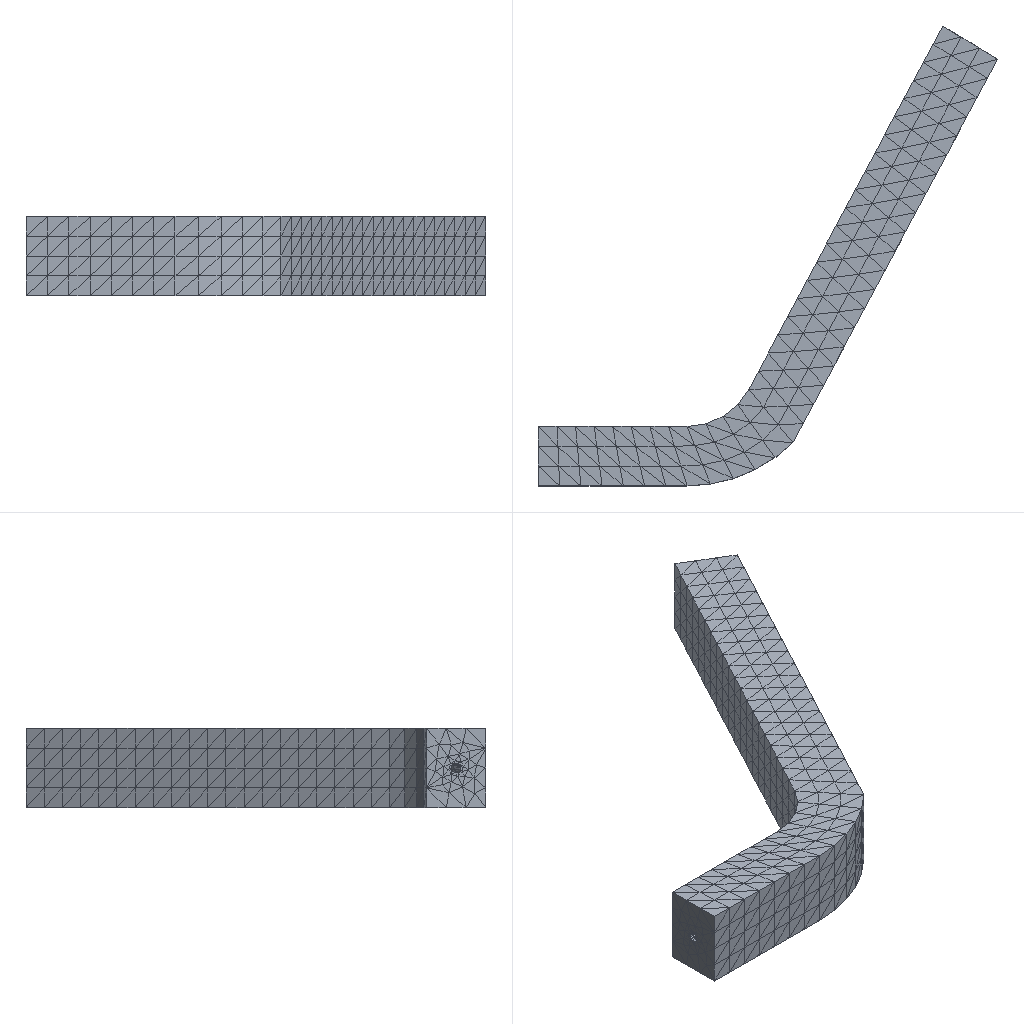Simulation study | abaqus
Set-up summary:
category,name,step,type,value,unit,region
solver,abaqus
solver,version,,,Abaqus/Standard 2020
units,not stated in the deck,,not stated
analysis,deck,,transient,transient
load_step,Step-1,Step-1,transient
load_step,requested,,,1
mesh,nodes,,,8863
mesh,elements,,,21207
element_type,S4R,,shell,2920
element_type,C3D4,,solid,16327
element_type,C3D8,,solid,1960
load,load commands in deck,,count,1
bc,support commands in deck,,count,2
material,CHONG,,in results
material,SOIL,,in results
material,TUBE,,in results
check,setup vs results,,match,"per instance, exact: element labels, types and connectivity; labels of the nodes the elements use; coordinates of those nodes at SINGLE_PRECISION in 2 of 3 instance(s)"
Abaqus input file, long lists of numbers shortened:
*Heading
** Job name: Job-1 Model name: Model-1
** Generated by: Abaqus/CAE 2020
*Preprint, echo=NO, model=NO, history=NO, contact=NO
**
** PARTS
**
*Part, name=chong
*Node
      1,   79.917,   70.314, -0.2075
      2,   79.947,   70.298,  -0.1153
** (2392 more lines like these left out)
*Element, type=C3D8
   1,  121,  214,  215,  138,    7,  100,  101,   24
   2,  122,  123,  146,  213,    8,    9,   32,   99
** (1958 more lines like these left out)
*Nset, nset=Set-1, generate
    1,  2394,     1
*Elset, elset=Set-1, generate
    1,  1960,     1
*Nset, nset=Set-2, generate
    1,  2394,     1
*Elset, elset=Set-2, generate
    1,  1960,     1
** Section: chong
*Solid Section, elset=Set-2, material=chong
,
*End Part
**
*Part, name=soil-delete
*Node
      1,   25.707,  -1.644,           8.
      2,          15.,          -6.,           8.
** (3537 more lines like these left out)
*Element, type=C3D4
    1,  226, 1737, 1738, 1739
    2, 1737, 1740,  438,  436
** (16325 more lines like these left out)
*Nset, nset=Set-1, generate
    1,  3539,     1
*Elset, elset=Set-1, generate
     1,  16327,      1
** Section: soil
*Solid Section, elset=Set-1, material=soil
,
*End Part
**
*Part, name=tube
*Node
      1,   38.406,   12.536, -0.4341
      2,   38.197,   12.672,          0.5
** (2928 more lines like these left out)
*Element, type=S4R
   1,    1,    7,  252,   14
   2,    7,    8,  253,  252
** (2918 more lines like these left out)
*Nset, nset=Set-1, generate
    1,  2930,     1
*Elset, elset=Set-1, generate
    1,  2920,     1
** Section: tube
*Shell Section, elset=Set-1, material=tube
0.01, 5
*End Part
**
**
** ASSEMBLY
**
*Assembly, name=Assembly
**
*Instance, name=soil-delete-1, part=soil-delete
*End Instance
**
*Instance, name=tube-1, part=tube
   -14.447,   -11.422,           4.
*End Instance
**
*Instance, name=chong-1, part=chong
  -36.883,   -33.511,           4.
*End Instance
**
*Node
      1,    43.596,   38.768,           4.
*Nset, nset=Set-1, instance=soil-delete-1
   1,   2,   3,   4,   9,  10,  14,  15,  23,  24,  25,  26,  27,  28,  29,  30
  31,  32,  33,  34,  35,  36,  49,  50,  51,  52,  53,  54,  55,  56,  57,  58
** (9 more lines like these left out)
*Elset, elset=Set-1, instance=soil-delete-1
    81,    98,   396,   701,   845,   892,  1273,  1789,  2345,  2356,  2379,  2423,  2521,  2581,  2591,  2592
  2622,  2642,  2644,  2646,  2669,  2680,  2683,  2695,  2700,  2711,  2712,  2724,  2729,  2745,  2747,  2760
** (14 more lines like these left out)
*Nset, nset=Set-2, instance=soil-delete-1
   1,   2,   3,   4,   5,   6,   7,   8,   9,  10,  11,  12,  13,  14,  15,  16
  23,  24,  25,  26,  30,  31,  32,  33,  37,  38,  39,  43,  44,  45,  49,  50
** (15 more lines like these left out)
*Elset, elset=Set-2, instance=soil-delete-1
    10,   141,   160,   634,   727,  2316,  2329,  2383,  2409,  2425,  2446,  2449,  2469,  2502,  2507,  2510
  2515,  2523,  2531,  2542,  2561,  2572,  2575,  2583,  2593,  2600,  2660,  2685,  2690,  2700,  2704,  2723
** (22 more lines like these left out)
*Nset, nset=Set-4
 1,
*Nset, nset=Set-7
 1,
*Nset, nset=Set-8
 1,
*Nset, nset=Set-9, instance=chong-1, generate
    1,  2394,     1
*Nset, nset=Set-9
 1,
*Elset, elset=Set-9, instance=chong-1, generate
    1,  1960,     1
*Nset, nset=Set-10, instance=chong-1, generate
 2281,  2394,     1
*Elset, elset=Set-10, instance=chong-1, generate
 1863,  1960,     1
*Nset, nset=b_Set-5, instance=chong-1, generate
    1,  2394,     1
*Elset, elset=b_Set-5, instance=chong-1, generate
    1,  1960,     1
*Nset, nset=m_Set-3
 1,
*Nset, nset=_PickedSet26, internal
 1,
*Elset, elset=_Surf-6_S1, internal, instance=chong-1, generate
 1863,  1960,     1
*Surface, type=ELEMENT, name=Surf-6
_Surf-6_S1, S1
*Elset, elset=_Surf-12_S1, internal, instance=chong-1, generate
 1863,  1960,     1
*Surface, type=ELEMENT, name=Surf-12
_Surf-12_S1, S1
*Elset, elset=_m_Surf-3_SPOS, internal, instance=tube-1, generate
    1,  2920,     1
*Surface, type=ELEMENT, name=m_Surf-3
_m_Surf-3_SPOS, SPOS
*Elset, elset=_m_Surf-7_S6, internal, instance=chong-1
    1,   15,   22,   24,   99,  113,  120,  122,  197,  211,  218,  220,  295,  309,  316,  318
  393,  407,  414,  416,  491,  505,  512,  514,  589,  603,  610,  612,  687,  701,  708,  710
** (3 more lines like these left out)
*Elset, elset=_m_Surf-7_S3, internal, instance=chong-1
    2,    3,    4,    9,   12,   21,   26,   27,   31,   33,   39,   40,   44,   88,   90,  100
  101,  102,  107,  110,  119,  124,  125,  129,  131,  137,  138,  142,  186,  188,  198,  199
** (17 more lines like these left out)
*Elset, elset=_m_Surf-7_S4, internal, instance=chong-1
    5,    6,   25,   43,   54,  103,  104,  123,  141,  152,  201,  202,  221,  239,  250,  299
  300,  319,  337,  348,  397,  398,  417,  435,  446,  495,  496,  515,  533,  544,  593,  594
** (5 more lines like these left out)
*Elset, elset=_m_Surf-7_S5, internal, instance=chong-1
   20,   23,   28,   46,   56,   57,  118,  121,  126,  144,  154,  155,  216,  219,  224,  242
  252,  253,  314,  317,  322,  340,  350,  351,  412,  415,  420,  438,  448,  449,  510,  513
** (6 more lines like these left out)
*Surface, type=ELEMENT, name=m_Surf-7
_m_Surf-7_S6, S6
_m_Surf-7_S3, S3
_m_Surf-7_S4, S4
_m_Surf-7_S5, S5
*Elset, elset=_m_Surf-9_S6, internal, instance=chong-1
    1,   15,   22,   24,   99,  113,  120,  122,  197,  211,  218,  220,  295,  309,  316,  318
  393,  407,  414,  416,  491,  505,  512,  514,  589,  603,  610,  612,  687,  701,  708,  710
** (3 more lines like these left out)
*Elset, elset=_m_Surf-9_S3, internal, instance=chong-1
    2,    3,    4,    9,   12,   21,   26,   27,   31,   33,   39,   40,   44,   88,   90,  100
  101,  102,  107,  110,  119,  124,  125,  129,  131,  137,  138,  142,  186,  188,  198,  199
** (17 more lines like these left out)
*Elset, elset=_m_Surf-9_S4, internal, instance=chong-1
    5,    6,   25,   43,   54,  103,  104,  123,  141,  152,  201,  202,  221,  239,  250,  299
  300,  319,  337,  348,  397,  398,  417,  435,  446,  495,  496,  515,  533,  544,  593,  594
** (5 more lines like these left out)
*Elset, elset=_m_Surf-9_S5, internal, instance=chong-1
   20,   23,   28,   46,   56,   57,  118,  121,  126,  144,  154,  155,  216,  219,  224,  242
  252,  253,  314,  317,  322,  340,  350,  351,  412,  415,  420,  438,  448,  449,  510,  513
** (6 more lines like these left out)
*Surface, type=ELEMENT, name=m_Surf-9
_m_Surf-9_S6, S6
_m_Surf-9_S3, S3
_m_Surf-9_S4, S4
_m_Surf-9_S5, S5
*Elset, elset=_s_Surf-1_S4, internal, instance=soil-delete-1
   353,   354,   411,   600,  1045,  1799,  2111,  2165,  2408,  2628,  2755,  3114,  3390,  3399,  3863,  4025
  4148,  4152,  4155,  4516,  4592,  4598,  4867,  4878,  5204,  5264,  5514,  5578,  5588,  5632,  5656,  5686
** (8 more lines like these left out)
*Elset, elset=_s_Surf-1_S3, internal, instance=soil-delete-1
   188,   220,   544,   547,   557,   573,   609,   667,   721,   772,   809,  1021,  1056,  1163,  1184,  1210
  1242,  1291,  1376,  1426,  1904,  1910,  1956,  2163,  2173,  2290,  2360,  2372,  2385,  2397,  2399,  2407
** (131 more lines like these left out)
*Elset, elset=_s_Surf-1_S2, internal, instance=soil-delete-1
   259,   452,   463,  1039,  2512,  2587,  3238,  3459,  4406,  4449,  4641,  5482,  5559,  5655,  5682,  5709
  5844,  5845,  5931,  5998,  6223,  6487,  6607,  6654,  6656,  6877,  6907,  6958,  7062,  7117,  7549,  7899
** (3 more lines like these left out)
*Elset, elset=_s_Surf-1_S1, internal, instance=soil-delete-1
   275,   592,   610,  1227,  1656,  1668,  2450,  2630,  2728,  2895,  3482,  3792,  4225,  4760,  5383,  5666
  5700,  5853,  6283,  6494,  6699,  6726,  6953,  7164,  7395,  7554,  7582,  7583,  7620,  7642,  7643,  7647
** (3 more lines like these left out)
*Surface, type=ELEMENT, name=s_Surf-1
_s_Surf-1_S4, S4
_s_Surf-1_S3, S3
_s_Surf-1_S2, S2
_s_Surf-1_S1, S1
*Elset, elset=_s_Surf-3_S4, internal, instance=soil-delete-1
   353,   354,   411,   600,  1045,  1799,  2111,  2165,  2408,  2628,  2755,  3114,  3390,  3399,  3863,  4025
  4148,  4152,  4155,  4516,  4592,  4598,  4867,  4878,  5204,  5264,  5514,  5578,  5588,  5632,  5656,  5686
** (8 more lines like these left out)
*Elset, elset=_s_Surf-3_S3, internal, instance=soil-delete-1
   188,   220,   544,   547,   557,   573,   609,   667,   721,   772,   809,  1021,  1056,  1163,  1184,  1210
  1242,  1291,  1376,  1426,  1904,  1910,  1956,  2163,  2173,  2290,  2360,  2372,  2385,  2397,  2399,  2407
** (131 more lines like these left out)
*Elset, elset=_s_Surf-3_S2, internal, instance=soil-delete-1
   259,   452,   463,  1039,  2512,  2587,  3238,  3459,  4406,  4449,  4641,  5482,  5559,  5655,  5682,  5709
  5844,  5845,  5931,  5998,  6223,  6487,  6607,  6654,  6656,  6877,  6907,  6958,  7062,  7117,  7549,  7899
** (3 more lines like these left out)
*Elset, elset=_s_Surf-3_S1, internal, instance=soil-delete-1
   275,   592,   610,  1227,  1656,  1668,  2450,  2630,  2728,  2895,  3482,  3792,  4225,  4760,  5383,  5666
  5700,  5853,  6283,  6494,  6699,  6726,  6953,  7164,  7395,  7554,  7582,  7583,  7620,  7642,  7643,  7647
** (3 more lines like these left out)
*Surface, type=ELEMENT, name=s_Surf-3
_s_Surf-3_S4, S4
_s_Surf-3_S3, S3
_s_Surf-3_S2, S2
_s_Surf-3_S1, S1
*Elset, elset=_s_Surf-5_S6, internal, instance=chong-1
    1,   15,   22,   24,   99,  113,  120,  122,  197,  211,  218,  220,  295,  309,  316,  318
  393,  407,  414,  416,  491,  505,  512,  514,  589,  603,  610,  612,  687,  701,  708,  710
** (3 more lines like these left out)
*Elset, elset=_s_Surf-5_S3, internal, instance=chong-1
    2,    3,    4,    9,   12,   21,   26,   27,   31,   33,   39,   40,   44,   88,   90,  100
  101,  102,  107,  110,  119,  124,  125,  129,  131,  137,  138,  142,  186,  188,  198,  199
** (17 more lines like these left out)
*Elset, elset=_s_Surf-5_S4, internal, instance=chong-1
    5,    6,   25,   43,   54,  103,  104,  123,  141,  152,  201,  202,  221,  239,  250,  299
  300,  319,  337,  348,  397,  398,  417,  435,  446,  495,  496,  515,  533,  544,  593,  594
** (5 more lines like these left out)
*Elset, elset=_s_Surf-5_S5, internal, instance=chong-1
   20,   23,   28,   46,   56,   57,  118,  121,  126,  144,  154,  155,  216,  219,  224,  242
  252,  253,  314,  317,  322,  340,  350,  351,  412,  415,  420,  438,  448,  449,  510,  513
** (6 more lines like these left out)
*Elset, elset=_s_Surf-5_S1, internal, instance=chong-1, generate
 1863,  1960,     1
*Elset, elset=_s_Surf-5_S2, internal, instance=chong-1, generate
  1,  98,   1
*Surface, type=ELEMENT, name=s_Surf-5
_s_Surf-5_S6, S6
_s_Surf-5_S3, S3
_s_Surf-5_S4, S4
_s_Surf-5_S2, S2
_s_Surf-5_S5, S5
_s_Surf-5_S1, S1
*Elset, elset=_s_Surf-7_SPOS, internal, instance=tube-1, generate
    1,  2920,     1
*Surface, type=ELEMENT, name=s_Surf-7
_s_Surf-7_SPOS, SPOS
*Elset, elset=_s_Surf-9_SPOS, internal, instance=tube-1, generate
    1,  2920,     1
*Surface, type=ELEMENT, name=s_Surf-9
_s_Surf-9_SPOS, SPOS
*Elset, elset=_s_Surf-11_S1, internal, instance=chong-1, generate
 1863,  1960,     1
*Surface, type=ELEMENT, name=s_Surf-11
_s_Surf-11_S1, S1
** Constraint: Constraint-1
*Tie, name=Constraint-1, adjust=yes
s_Surf-3, m_Surf-3
*End Assembly
**
** MATERIALS
**
*Material, name=chong
*Density
1050.,
*Elastic
 8e+06, 0.49
*Material, name=soil
*Density
2000.,
*Elastic
 3e+07, 0.3
*Material, name=tube
*Density
7800.,
*Elastic
 2.06e+11, 0.25
**
** INTERACTION PROPERTIES
**
*Surface Interaction, name=IntProp-1
1.,
*Friction, slip tolerance=0.005
 0.01,
*Surface Behavior, pressure-overclosure=HARD
**
** BOUNDARY CONDITIONS
**
** Name: BC-1 Type: 对称/反对称/完全固定
*Boundary
Set-1, ENCASTRE
** Name: BC-2 Type: 位移/转角
*Boundary
Set-2, 3, 3
**
** INTERACTIONS
**
** Interaction: Int-2
*Contact Pair, interaction=IntProp-1, type=SURFACE TO SURFACE
s_Surf-9, m_Surf-9
** ----------------------------------------------------------------
**
** STEP: Step-1
**
*Step, name=Step-1, nlgeom=YES, inc=1000
*Dynamic
0.001,3.,0.0005
**
** LOADS
**
** Name: Load-1   Type: Pressure
*Dsload
Surf-12, P, 140000.
**
** CONTROLS
**
*Controls, reset
*Controls, parameters=time incrementation
, , , , , , , 20, , ,
**
** OUTPUT REQUESTS
**
*Restart, write, number interval=1, time marks=NO
**
** FIELD OUTPUT: F-Output-1
**
*Output, field, frequency=1
*Node Output
RF, U, V
*Element Output, directions=YES
E, LE, MISES, PE, PEEQ, S
*Contact Output
CDISP, CFORCE, CSTRESS
**
** HISTORY OUTPUT: H-Output-1
**
*Output, history, variable=PRESELECT, number interval=200, time marks=NO
*End Step
Results summary:
result,step,,completed,increments=65 time=3.0/3.0
result,analysis,,,transient
result,last_loadstep,,,1
result,primary field,,,"U, UR"
result,reaction total,,FX,3e-05,model units
result,reaction total,,FY,-2.9e-05,model units
result,reaction total,,FZ,-1e-06,model units